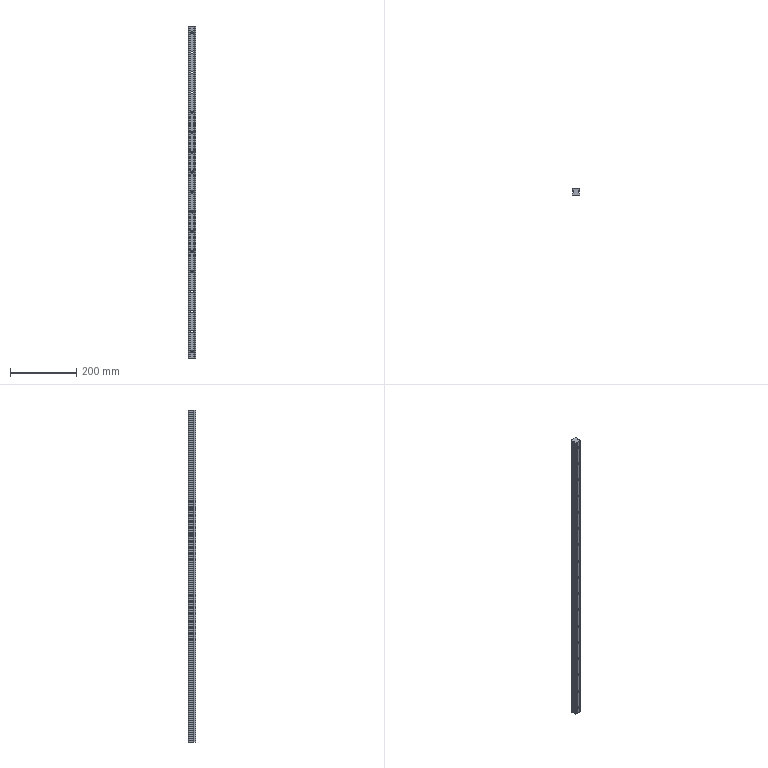Part | STEP file | HGH 25HA-950 | 1 solid | 119 faces | box 23 x 22 x 1000 mm | volume 420521 mm3 | cylinder 72 | plane 47 | commonest cylinder face diameters 6.6 x34 11 x34 4.6 x4